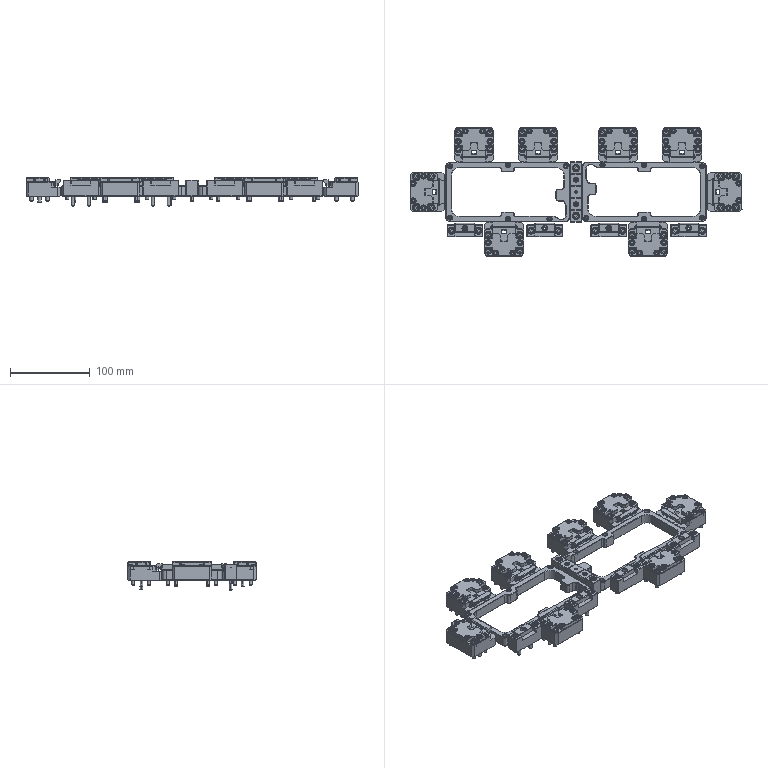Part | SolidWorks | features Attribute 1 | 181 solids | 6400 faces | volume 446882 mm3 | plane 2788 | cylinder 1648 | cone 1300 | torus 552 | sphere 112 | commonest cylinder face diameters 4 x284 3 x274 2 x168 6.5 x132 4.5 x88 5.5 x88